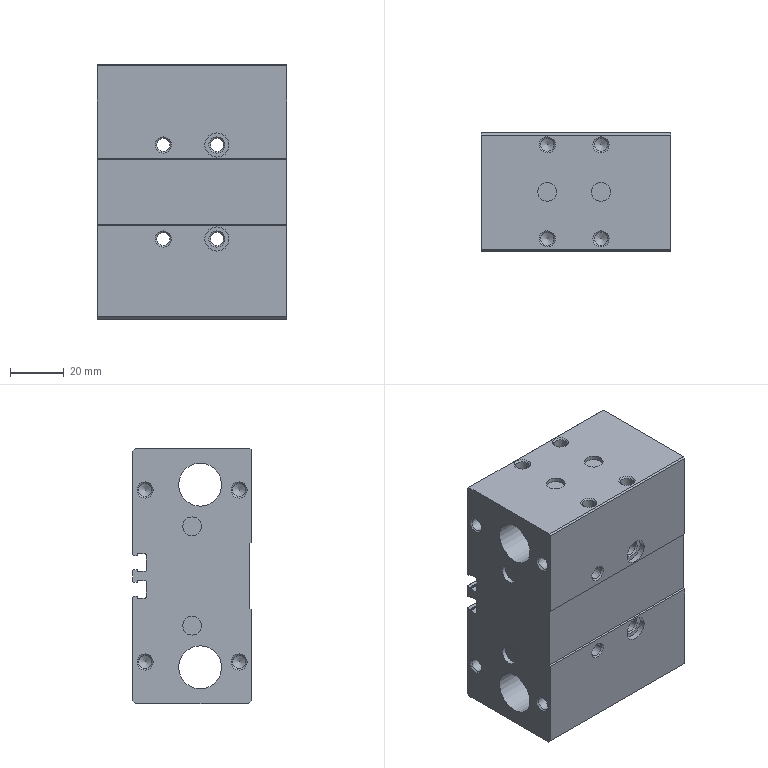Part | NX | features BREP 1 | 1 solid | 126 faces | box 70.6 x 44.05 x 95 mm | volume 227497 mm3 | plane 51 | cylinder 51 | cone 24 | commonest cylinder face diameters 4.917 x12 0.4 x8 0.8 x8 9 x6 5.2 x4 7 x4